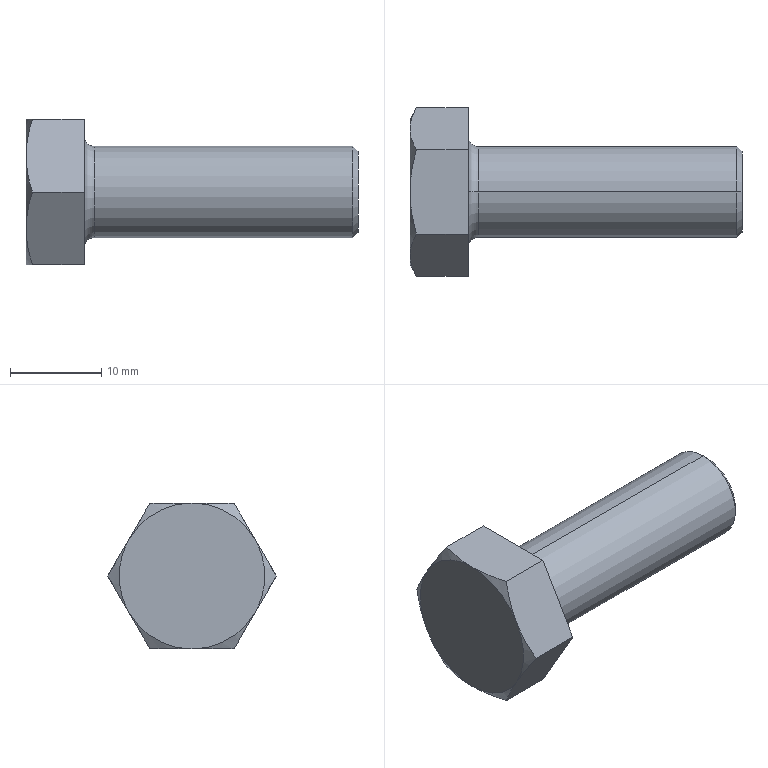Part | SolidWorks | features Chamfer 2, RevCut 2, Revolution 2, Extrusion 1, ICE 1 | 1 solid | 21 faces | box 36.4 x 18.475 x 16 mm | volume 3775 mm3 | plane 9 | cone 8 | cylinder 2 | torus 2 | commonest cylinder face diameters 10 x2
STEP:
#1=CARTESIAN_POINT('',(36.4,0.,-4.444));
#2=VERTEX_POINT('',#1);
#3=CARTESIAN_POINT('',(36.4,0.,4.444));
#4=VERTEX_POINT('',#3);
#5=CARTESIAN_POINT('',(36.4,0.,0.));
#6=DIRECTION('',(1.,0.,0.));
#7=DIRECTION('',(0.,0.,1.));
#8=AXIS2_PLACEMENT_3D('',#5,#6,#7);
#9=CIRCLE('',#8,4.444);
#10=EDGE_CURVE('',#2,#4,#9,.T.);
#11=ORIENTED_EDGE('',*,*,#10,.F.);
#12=CARTESIAN_POINT('',(35.844,0.,-5.));
#13=VERTEX_POINT('',#12);
#14=CARTESIAN_POINT('',(35.844,0.,-5.));
#15=DIRECTION('',(-0.7071,0.,-0.7071));
#16=VECTOR('',#15,1000.);
#17=LINE('',#14,#16);
#18=EDGE_CURVE('',#2,#13,#17,.T.);
#19=ORIENTED_EDGE('',*,*,#18,.T.);
#20=CARTESIAN_POINT('',(35.844,0.,5.));
#21=VERTEX_POINT('',#20);
#22=CARTESIAN_POINT('',(35.844,0.,0.));
#23=DIRECTION('',(-1.,0.,0.));
#24=DIRECTION('',(0.,0.,1.));
#25=AXIS2_PLACEMENT_3D('',#22,#23,#24);
#26=CIRCLE('',#25,5.);
#27=EDGE_CURVE('',#21,#13,#26,.T.);
#28=ORIENTED_EDGE('',*,*,#27,.F.);
#29=CARTESIAN_POINT('',(35.844,0.,5.));
#30=DIRECTION('',(-0.7071,0.,0.7071));
#31=VECTOR('',#30,1000.);
#32=LINE('',#29,#31);
#33=EDGE_CURVE('',#4,#21,#32,.T.);
#34=ORIENTED_EDGE('',*,*,#33,.F.);
#35=EDGE_LOOP('',(#11,#19,#28,#34));
#36=FACE_OUTER_BOUND('',#35,.T.);
#37=CARTESIAN_POINT('',(35.844,0.,0.));
#38=DIRECTION('',(-1.,0.,0.));
#39=DIRECTION('',(0.,0.,1.));
#40=AXIS2_PLACEMENT_3D('',#37,#38,#39);
#41=CONICAL_SURFACE('',#40,5.,0.7854);
#42=ADVANCED_FACE('',(#36),#41,.T.);
#43=ORIENTED_EDGE('',*,*,#27,.T.);
#44=CARTESIAN_POINT('',(7.5,0.,-5.));
#45=VERTEX_POINT('',#44);
#46=CARTESIAN_POINT('',(6.4,0.,-5.));
#47=DIRECTION('',(-1.,0.,0.));
#48=VECTOR('',#47,1000.);
#49=LINE('',#46,#48);
#50=EDGE_CURVE('',#13,#45,#49,.T.);
#51=ORIENTED_EDGE('',*,*,#50,.T.);
#52=CARTESIAN_POINT('',(7.5,0.,5.));
#53=VERTEX_POINT('',#52);
#54=CARTESIAN_POINT('',(7.5,0.,0.));
#55=DIRECTION('',(-1.,0.,0.));
#56=DIRECTION('',(0.,0.,1.));
#57=AXIS2_PLACEMENT_3D('',#54,#55,#56);
#58=CIRCLE('',#57,5.);
#59=EDGE_CURVE('',#53,#45,#58,.T.);
#60=ORIENTED_EDGE('',*,*,#59,.F.);
#61=CARTESIAN_POINT('',(6.4,0.,5.));
#62=DIRECTION('',(-1.,0.,0.));
#63=VECTOR('',#62,1000.);
#64=LINE('',#61,#63);
#65=EDGE_CURVE('',#21,#53,#64,.T.);
#66=ORIENTED_EDGE('',*,*,#65,.F.);
#67=EDGE_LOOP('',(#43,#51,#60,#66));
#68=FACE_OUTER_BOUND('',#67,.T.);
#69=CARTESIAN_POINT('',(6.4,0.,0.));
#70=DIRECTION('',(-1.,0.,0.));
#71=DIRECTION('',(0.,0.,1.));
#72=AXIS2_PLACEMENT_3D('',#69,#70,#71);
#73=CYLINDRICAL_SURFACE('',#72,5.);
#74=ADVANCED_FACE('',(#68),#73,.T.);
#75=CARTESIAN_POINT('',(6.4,0.,-6.1));
#76=VERTEX_POINT('',#75);
#77=CARTESIAN_POINT('',(6.4,0.,6.1));
#78=VERTEX_POINT('',#77);
#79=CARTESIAN_POINT('',(6.4,0.,0.));
#80=DIRECTION('',(-1.,0.,0.));
#81=DIRECTION('',(0.,0.,1.));
#82=AXIS2_PLACEMENT_3D('',#79,#80,#81);
#83=CIRCLE('',#82,6.1);
#84=EDGE_CURVE('',#76,#78,#83,.T.);
#85=ORIENTED_EDGE('',*,*,#84,.F.);
#86=CARTESIAN_POINT('',(7.5,0.,-6.1));
#87=DIRECTION('',(0.,1.,0.));
#88=DIRECTION('',(0.,0.,1.));
#89=AXIS2_PLACEMENT_3D('',#86,#87,#88);
#90=CIRCLE('',#89,1.1);
#91=EDGE_CURVE('',#76,#45,#90,.T.);
#92=ORIENTED_EDGE('',*,*,#91,.T.);
#93=CARTESIAN_POINT('',(7.5,0.,0.));
#94=DIRECTION('',(-1.,0.,0.));
#95=DIRECTION('',(0.,0.,1.));
#96=AXIS2_PLACEMENT_3D('',#93,#94,#95);
#97=CIRCLE('',#96,5.);
#98=EDGE_CURVE('',#45,#53,#97,.T.);
#99=ORIENTED_EDGE('',*,*,#98,.T.);
#100=CARTESIAN_POINT('',(7.5,0.,6.1));
#101=DIRECTION('',(0.,-1.,0.));
#102=DIRECTION('',(0.,0.,-1.));
#103=AXIS2_PLACEMENT_3D('',#100,#101,#102);
#104=CIRCLE('',#103,1.1);
#105=EDGE_CURVE('',#78,#53,#104,.T.);
#106=ORIENTED_EDGE('',*,*,#105,.F.);
#107=EDGE_LOOP('',(#85,#92,#99,#106));
#108=FACE_OUTER_BOUND('',#107,.T.);
#109=CARTESIAN_POINT('',(7.5,0.,0.));
#110=DIRECTION('',(-1.,0.,0.));
#111=DIRECTION('',(0.,0.,1.));
#112=AXIS2_PLACEMENT_3D('',#109,#110,#111);
#113=TOROIDAL_SURFACE('',#112,6.1,1.1);
#114=ADVANCED_FACE('',(#108),#113,.F.);
#115=CARTESIAN_POINT('',(6.4,-4.619,-8.));
#116=VERTEX_POINT('',#115);
#117=CARTESIAN_POINT('',(6.4,4.619,-8.));
#118=VERTEX_POINT('',#117);
#119=CARTESIAN_POINT('',(6.4,-4.619,-8.));
#120=DIRECTION('',(0.,1.,0.));
#121=VECTOR('',#120,1000.);
#122=LINE('',#119,#121);
#123=EDGE_CURVE('',#116,#118,#122,.T.);
#124=ORIENTED_EDGE('',*,*,#123,.T.);
#125=CARTESIAN_POINT('',(6.4,9.238,0.));
#126=VERTEX_POINT('',#125);
#127=CARTESIAN_POINT('',(6.4,4.619,-8.));
#128=DIRECTION('',(0.,0.5,0.866));
#129=VECTOR('',#128,1000.);
#130=LINE('',#127,#129);
#131=EDGE_CURVE('',#118,#126,#130,.T.);
#132=ORIENTED_EDGE('',*,*,#131,.T.);
#133=CARTESIAN_POINT('',(6.4,4.619,8.));
#134=VERTEX_POINT('',#133);
#135=CARTESIAN_POINT('',(6.4,9.238,0.));
#136=DIRECTION('',(0.,-0.5,0.866));
#137=VECTOR('',#136,1000.);
#138=LINE('',#135,#137);
#139=EDGE_CURVE('',#126,#134,#138,.T.);
#140=ORIENTED_EDGE('',*,*,#139,.T.);
#141=CARTESIAN_POINT('',(6.4,-4.619,8.));
#142=VERTEX_POINT('',#141);
#143=CARTESIAN_POINT('',(6.4,4.619,8.));
#144=DIRECTION('',(0.,-1.,0.));
#145=VECTOR('',#144,1000.);
#146=LINE('',#143,#145);
#147=EDGE_CURVE('',#134,#142,#146,.T.);
#148=ORIENTED_EDGE('',*,*,#147,.T.);
#149=CARTESIAN_POINT('',(6.4,-9.238,0.));
#150=VERTEX_POINT('',#149);
#151=CARTESIAN_POINT('',(6.4,-4.619,8.));
#152=DIRECTION('',(0.,-0.5,-0.866));
#153=VECTOR('',#152,1000.);
#154=LINE('',#151,#153);
#155=EDGE_CURVE('',#142,#150,#154,.T.);
#156=ORIENTED_EDGE('',*,*,#155,.T.);
#157=CARTESIAN_POINT('',(6.4,-9.238,0.));
#158=DIRECTION('',(0.,0.5,-0.866));
#159=VECTOR('',#158,1000.);
#160=LINE('',#157,#159);
#161=EDGE_CURVE('',#150,#116,#160,.T.);
#162=ORIENTED_EDGE('',*,*,#161,.T.);
#163=EDGE_LOOP('',(#124,#132,#140,#148,#156,#162));
#164=FACE_OUTER_BOUND('',#163,.T.);
#165=CARTESIAN_POINT('',(6.4,0.,0.));
#166=DIRECTION('',(-1.,0.,0.));
#167=DIRECTION('',(0.,0.,1.));
#168=AXIS2_PLACEMENT_3D('',#165,#166,#167);
#169=CIRCLE('',#168,6.1);
#170=EDGE_CURVE('',#78,#76,#169,.T.);
#171=ORIENTED_EDGE('',*,*,#170,.T.);
#172=ORIENTED_EDGE('',*,*,#84,.T.);
#173=EDGE_LOOP('',(#171,#172));
#174=FACE_BOUND('',#173,.T.);
#175=CARTESIAN_POINT('',(6.4,4.619,-8.));
#176=DIRECTION('',(1.,0.,0.));
#177=DIRECTION('',(0.,0.,-1.));
#178=AXIS2_PLACEMENT_3D('',#175,#176,#177);
#179=PLANE('',#178);
#180=ADVANCED_FACE('',(#164,#174),#179,.T.);
#181=CARTESIAN_POINT('',(0.7145,4.619,-8.));
#182=VERTEX_POINT('',#181);
#183=CARTESIAN_POINT('',(0.,0.,-8.));
#184=VERTEX_POINT('',#183);
#185=CARTESIAN_POINT('',(0.7145,4.619,-8.));
#186=CARTESIAN_POINT('',(0.4989,3.872,-8.));
#187=CARTESIAN_POINT('',(0.3194,3.115,-8.));
#188=CARTESIAN_POINT('',(0.06895,1.573,-8.));
#189=CARTESIAN_POINT('',(0.,0.781,-8.));
#190=CARTESIAN_POINT('',(0.,0.,-8.));
#191=B_SPLINE_CURVE_WITH_KNOTS('',3,(#185,#186,#187,#188,#189,#190),.UNSPECIFIED.,.F.,.F.,(4,2,4),(0.003372,0.005703,0.008035),.UNSPECIFIED.);
#192=EDGE_CURVE('',#182,#184,#191,.T.);
#193=ORIENTED_EDGE('',*,*,#192,.F.);
#194=CARTESIAN_POINT('',(6.4,4.619,-8.));
#195=DIRECTION('',(-1.,0.,0.));
#196=VECTOR('',#195,1000.);
#197=LINE('',#194,#196);
#198=EDGE_CURVE('',#118,#182,#197,.T.);
#199=ORIENTED_EDGE('',*,*,#198,.F.);
#200=ORIENTED_EDGE('',*,*,#123,.F.);
#201=CARTESIAN_POINT('',(0.7145,-4.619,-8.));
#202=VERTEX_POINT('',#201);
#203=CARTESIAN_POINT('',(6.4,-4.619,-8.));
#204=DIRECTION('',(-1.,0.,0.));
#205=VECTOR('',#204,1000.);
#206=LINE('',#203,#205);
#207=EDGE_CURVE('',#116,#202,#206,.T.);
#208=ORIENTED_EDGE('',*,*,#207,.T.);
#209=CARTESIAN_POINT('',(0.,0.,-8.));
#210=CARTESIAN_POINT('',(0.,-0.7805,-8.));
#211=CARTESIAN_POINT('',(0.06709,-1.556,-8.));
#212=CARTESIAN_POINT('',(0.3158,-3.098,-8.));
#213=CARTESIAN_POINT('',(0.4977,-3.868,-8.));
#214=CARTESIAN_POINT('',(0.7145,-4.619,-8.));
#215=B_SPLINE_CURVE_WITH_KNOTS('',3,(#209,#210,#211,#212,#213,#214),.UNSPECIFIED.,.F.,.F.,(4,2,4),(0.008035,0.01037,0.0127),.UNSPECIFIED.);
#216=EDGE_CURVE('',#184,#202,#215,.T.);
#217=ORIENTED_EDGE('',*,*,#216,.F.);
#218=EDGE_LOOP('',(#193,#199,#200,#208,#217));
#219=FACE_OUTER_BOUND('',#218,.T.);
#220=CARTESIAN_POINT('',(6.4,-4.619,-8.));
#221=DIRECTION('',(0.,0.,1.));
#222=DIRECTION('',(1.,0.,0.));
#223=AXIS2_PLACEMENT_3D('',#220,#221,#222);
#224=PLANE('',#223);
#225=ADVANCED_FACE('',(#219),#224,.F.);
#226=CARTESIAN_POINT('',(0.7145,9.238,0.));
#227=VERTEX_POINT('',#226);
#228=CARTESIAN_POINT('',(0.,6.928,-4.));
#229=VERTEX_POINT('',#228);
#230=CARTESIAN_POINT('',(0.7145,9.238,0.));
#231=CARTESIAN_POINT('',(0.4964,8.86,-0.6543));
#232=CARTESIAN_POINT('',(0.3167,8.479,-1.313));
#233=CARTESIAN_POINT('',(0.0681,7.71,-2.646));
#234=CARTESIAN_POINT('',(0.,7.322,-3.319));
#235=CARTESIAN_POINT('',(0.,6.928,-4.));
#236=B_SPLINE_CURVE_WITH_KNOTS('',3,(#230,#231,#232,#233,#234,#235),.UNSPECIFIED.,.F.,.F.,(4,2,4),(0.000000238,0.002337,0.004674),.UNSPECIFIED.);
#237=EDGE_CURVE('',#227,#229,#236,.T.);
#238=ORIENTED_EDGE('',*,*,#237,.F.);
#239=CARTESIAN_POINT('',(6.4,9.238,0.));
#240=DIRECTION('',(-1.,0.,0.));
#241=VECTOR('',#240,1000.);
#242=LINE('',#239,#241);
#243=EDGE_CURVE('',#126,#227,#242,.T.);
#244=ORIENTED_EDGE('',*,*,#243,.F.);
#245=ORIENTED_EDGE('',*,*,#131,.F.);
#246=ORIENTED_EDGE('',*,*,#198,.T.);
#247=CARTESIAN_POINT('',(0.,6.928,-4.));
#248=CARTESIAN_POINT('',(0.,6.732,-4.339));
#249=CARTESIAN_POINT('',(0.01689,6.535,-4.68));
#250=CARTESIAN_POINT('',(0.08225,6.146,-5.355));
#251=CARTESIAN_POINT('',(0.1307,5.952,-5.69));
#252=CARTESIAN_POINT('',(0.3174,5.376,-6.689));
#253=CARTESIAN_POINT('',(0.497,4.996,-7.347));
#254=CARTESIAN_POINT('',(0.7145,4.619,-8.));
#255=B_SPLINE_CURVE_WITH_KNOTS('',3,(#247,#248,#249,#250,#251,#252,#253,#254),.UNSPECIFIED.,.F.,.F.,(4,2,2,4),(0.004674,0.005838,0.007002,0.00933),.UNSPECIFIED.);
#256=EDGE_CURVE('',#229,#182,#255,.T.);
#257=ORIENTED_EDGE('',*,*,#256,.F.);
#258=EDGE_LOOP('',(#238,#244,#245,#246,#257));
#259=FACE_OUTER_BOUND('',#258,.T.);
#260=CARTESIAN_POINT('',(6.4,4.619,-8.));
#261=DIRECTION('',(0.,-0.866,0.5));
#262=DIRECTION('',(0.,-0.5,-0.866));
#263=AXIS2_PLACEMENT_3D('',#260,#261,#262);
#264=PLANE('',#263);
#265=ADVANCED_FACE('',(#259),#264,.F.);
#266=CARTESIAN_POINT('',(0.7145,4.619,8.));
#267=VERTEX_POINT('',#266);
#268=CARTESIAN_POINT('',(0.,6.928,4.));
#269=VERTEX_POINT('',#268);
#270=CARTESIAN_POINT('',(0.7145,4.619,8.));
#271=CARTESIAN_POINT('',(0.4964,4.997,7.346));
#272=CARTESIAN_POINT('',(0.3167,5.377,6.687));
#273=CARTESIAN_POINT('',(0.0681,6.146,5.354));
#274=CARTESIAN_POINT('',(0.,6.535,4.681));
#275=CARTESIAN_POINT('',(0.,6.928,4.));
#276=B_SPLINE_CURVE_WITH_KNOTS('',3,(#270,#271,#272,#273,#274,#275),.UNSPECIFIED.,.F.,.F.,(4,2,4),(0.000000238,0.002337,0.004674),.UNSPECIFIED.);
#277=EDGE_CURVE('',#267,#269,#276,.T.);
#278=ORIENTED_EDGE('',*,*,#277,.F.);
#279=CARTESIAN_POINT('',(6.4,4.619,8.));
#280=DIRECTION('',(-1.,0.,0.));
#281=VECTOR('',#280,1000.);
#282=LINE('',#279,#281);
#283=EDGE_CURVE('',#134,#267,#282,.T.);
#284=ORIENTED_EDGE('',*,*,#283,.F.);
#285=ORIENTED_EDGE('',*,*,#139,.F.);
#286=ORIENTED_EDGE('',*,*,#243,.T.);
#287=CARTESIAN_POINT('',(0.,6.928,4.));
#288=CARTESIAN_POINT('',(0.,7.124,3.661));
#289=CARTESIAN_POINT('',(0.01689,7.321,3.32));
#290=CARTESIAN_POINT('',(0.08225,7.711,2.645));
#291=CARTESIAN_POINT('',(0.1307,7.904,2.31));
#292=CARTESIAN_POINT('',(0.3174,8.481,1.311));
#293=CARTESIAN_POINT('',(0.497,8.861,0.6527));
#294=CARTESIAN_POINT('',(0.7145,9.238,0.));
#295=B_SPLINE_CURVE_WITH_KNOTS('',3,(#287,#288,#289,#290,#291,#292,#293,#294),.UNSPECIFIED.,.F.,.F.,(4,2,2,4),(0.004674,0.005838,0.007002,0.00933),.UNSPECIFIED.);
#296=EDGE_CURVE('',#269,#227,#295,.T.);
#297=ORIENTED_EDGE('',*,*,#296,.F.);
#298=EDGE_LOOP('',(#278,#284,#285,#286,#297));
#299=FACE_OUTER_BOUND('',#298,.T.);
#300=CARTESIAN_POINT('',(6.4,9.238,0.));
#301=DIRECTION('',(0.,-0.866,-0.5));
#302=DIRECTION('',(0.,0.5,-0.866));
#303=AXIS2_PLACEMENT_3D('',#300,#301,#302);
#304=PLANE('',#303);
#305=ADVANCED_FACE('',(#299),#304,.F.);
#306=CARTESIAN_POINT('',(0.7145,-4.619,8.));
#307=VERTEX_POINT('',#306);
#308=CARTESIAN_POINT('',(0.,0.,8.));
#309=VERTEX_POINT('',#308);
#310=CARTESIAN_POINT('',(0.7145,-4.619,8.));
#311=CARTESIAN_POINT('',(0.4977,-3.868,8.));
#312=CARTESIAN_POINT('',(0.3158,-3.098,8.));
#313=CARTESIAN_POINT('',(0.06709,-1.556,8.));
#314=CARTESIAN_POINT('',(0.,-0.7805,8.));
#315=CARTESIAN_POINT('',(0.,0.,8.));
#316=B_SPLINE_CURVE_WITH_KNOTS('',3,(#310,#311,#312,#313,#314,#315),.UNSPECIFIED.,.F.,.F.,(4,2,4),(0.008254,0.01059,0.01293),.UNSPECIFIED.);
#317=EDGE_CURVE('',#307,#309,#316,.T.);
#318=ORIENTED_EDGE('',*,*,#317,.F.);
#319=CARTESIAN_POINT('',(6.4,-4.619,8.));
#320=DIRECTION('',(-1.,0.,0.));
#321=VECTOR('',#320,1000.);
#322=LINE('',#319,#321);
#323=EDGE_CURVE('',#142,#307,#322,.T.);
#324=ORIENTED_EDGE('',*,*,#323,.F.);
#325=ORIENTED_EDGE('',*,*,#147,.F.);
#326=ORIENTED_EDGE('',*,*,#283,.T.);
#327=CARTESIAN_POINT('',(0.,0.,8.));
#328=CARTESIAN_POINT('',(0.,0.781,8.));
#329=CARTESIAN_POINT('',(0.06895,1.573,8.));
#330=CARTESIAN_POINT('',(0.3194,3.115,8.));
#331=CARTESIAN_POINT('',(0.4989,3.872,8.));
#332=CARTESIAN_POINT('',(0.7145,4.619,8.));
#333=B_SPLINE_CURVE_WITH_KNOTS('',3,(#327,#328,#329,#330,#331,#332),.UNSPECIFIED.,.F.,.F.,(4,2,4),(0.01293,0.01526,0.0176),.UNSPECIFIED.);
#334=EDGE_CURVE('',#309,#267,#333,.T.);
#335=ORIENTED_EDGE('',*,*,#334,.F.);
#336=EDGE_LOOP('',(#318,#324,#325,#326,#335));
#337=FACE_OUTER_BOUND('',#336,.T.);
#338=CARTESIAN_POINT('',(6.4,4.619,8.));
#339=DIRECTION('',(0.,0.,-1.));
#340=DIRECTION('',(0.,1.,0.));
#341=AXIS2_PLACEMENT_3D('',#338,#339,#340);
#342=PLANE('',#341);
#343=ADVANCED_FACE('',(#337),#342,.F.);
#344=CARTESIAN_POINT('',(0.7145,-9.238,0.));
#345=VERTEX_POINT('',#344);
#346=CARTESIAN_POINT('',(0.,-6.928,4.));
#347=VERTEX_POINT('',#346);
#348=CARTESIAN_POINT('',(0.7145,-9.238,0.));
#349=CARTESIAN_POINT('',(0.4964,-8.86,0.6543));
#350=CARTESIAN_POINT('',(0.3167,-8.479,1.313));
#351=CARTESIAN_POINT('',(0.0681,-7.71,2.646));
#352=CARTESIAN_POINT('',(0.,-7.322,3.319));
#353=CARTESIAN_POINT('',(0.,-6.928,4.));
#354=B_SPLINE_CURVE_WITH_KNOTS('',3,(#348,#349,#350,#351,#352,#353),.UNSPECIFIED.,.F.,.F.,(4,2,4),(0.000000238,0.002337,0.004674),.UNSPECIFIED.);
#355=EDGE_CURVE('',#345,#347,#354,.T.);
#356=ORIENTED_EDGE('',*,*,#355,.F.);
#357=CARTESIAN_POINT('',(6.4,-9.238,0.));
#358=DIRECTION('',(-1.,0.,0.));
#359=VECTOR('',#358,1000.);
#360=LINE('',#357,#359);
#361=EDGE_CURVE('',#150,#345,#360,.T.);
#362=ORIENTED_EDGE('',*,*,#361,.F.);
#363=ORIENTED_EDGE('',*,*,#155,.F.);
#364=ORIENTED_EDGE('',*,*,#323,.T.);
#365=CARTESIAN_POINT('',(0.,-6.928,4.));
#366=CARTESIAN_POINT('',(0.,-6.732,4.339));
#367=CARTESIAN_POINT('',(0.01689,-6.535,4.68));
#368=CARTESIAN_POINT('',(0.08225,-6.146,5.355));
#369=CARTESIAN_POINT('',(0.1307,-5.952,5.69));
#370=CARTESIAN_POINT('',(0.3174,-5.376,6.689));
#371=CARTESIAN_POINT('',(0.497,-4.996,7.347));
#372=CARTESIAN_POINT('',(0.7145,-4.619,8.));
#373=B_SPLINE_CURVE_WITH_KNOTS('',3,(#365,#366,#367,#368,#369,#370,#371,#372),.UNSPECIFIED.,.F.,.F.,(4,2,2,4),(0.004674,0.005838,0.007002,0.00933),.UNSPECIFIED.);
#374=EDGE_CURVE('',#347,#307,#373,.T.);
#375=ORIENTED_EDGE('',*,*,#374,.F.);
#376=EDGE_LOOP('',(#356,#362,#363,#364,#375));
#377=FACE_OUTER_BOUND('',#376,.T.);
#378=CARTESIAN_POINT('',(6.4,-4.619,8.));
#379=DIRECTION('',(0.,0.866,-0.5));
#380=DIRECTION('',(0.,0.5,0.866));
#381=AXIS2_PLACEMENT_3D('',#378,#379,#380);
#382=PLANE('',#381);
#383=ADVANCED_FACE('',(#377),#382,.F.);
#384=CARTESIAN_POINT('',(0.,-6.928,-4.));
#385=VERTEX_POINT('',#384);
#386=CARTESIAN_POINT('',(0.7145,-4.619,-8.));
#387=CARTESIAN_POINT('',(0.4964,-4.997,-7.346));
#388=CARTESIAN_POINT('',(0.3167,-5.377,-6.687));
#389=CARTESIAN_POINT('',(0.0681,-6.146,-5.354));
#390=CARTESIAN_POINT('',(0.,-6.535,-4.681));
#391=CARTESIAN_POINT('',(0.,-6.928,-4.));
#392=B_SPLINE_CURVE_WITH_KNOTS('',3,(#386,#387,#388,#389,#390,#391),.UNSPECIFIED.,.F.,.F.,(4,2,4),(0.000000238,0.002337,0.004674),.UNSPECIFIED.);
#393=EDGE_CURVE('',#202,#385,#392,.T.);
#394=ORIENTED_EDGE('',*,*,#393,.F.);
#395=ORIENTED_EDGE('',*,*,#207,.F.);
#396=ORIENTED_EDGE('',*,*,#161,.F.);
#397=ORIENTED_EDGE('',*,*,#361,.T.);
#398=CARTESIAN_POINT('',(0.,-6.928,-4.));
#399=CARTESIAN_POINT('',(0.,-7.124,-3.661));
#400=CARTESIAN_POINT('',(0.01689,-7.321,-3.32));
#401=CARTESIAN_POINT('',(0.08225,-7.711,-2.645));
#402=CARTESIAN_POINT('',(0.1307,-7.904,-2.31));
#403=CARTESIAN_POINT('',(0.3174,-8.481,-1.311));
#404=CARTESIAN_POINT('',(0.497,-8.861,-0.6527));
#405=CARTESIAN_POINT('',(0.7145,-9.238,0.));
#406=B_SPLINE_CURVE_WITH_KNOTS('',3,(#398,#399,#400,#401,#402,#403,#404,#405),.UNSPECIFIED.,.F.,.F.,(4,2,2,4),(0.004674,0.005838,0.007002,0.00933),.UNSPECIFIED.);
#407=EDGE_CURVE('',#385,#345,#406,.T.);
#408=ORIENTED_EDGE('',*,*,#407,.F.);
#409=EDGE_LOOP('',(#394,#395,#396,#397,#408));
#410=FACE_OUTER_BOUND('',#409,.T.);
#411=CARTESIAN_POINT('',(6.4,-9.238,0.));
#412=DIRECTION('',(0.,0.866,0.5));
#413=DIRECTION('',(0.,-0.5,0.866));
#414=AXIS2_PLACEMENT_3D('',#411,#412,#413);
#415=PLANE('',#414);
#416=ADVANCED_FACE('',(#410),#415,.F.);
#417=ORIENTED_EDGE('',*,*,#216,.T.);
#418=ORIENTED_EDGE('',*,*,#393,.T.);
#419=CARTESIAN_POINT('',(0.,0.,0.));
#420=DIRECTION('',(1.,0.,0.));
#421=DIRECTION('',(0.,0.,-1.));
#422=AXIS2_PLACEMENT_3D('',#419,#420,#421);
#423=CIRCLE('',#422,8.);
#424=EDGE_CURVE('',#385,#184,#423,.T.);
#425=ORIENTED_EDGE('',*,*,#424,.T.);
#426=EDGE_LOOP('',(#417,#418,#425));
#427=FACE_OUTER_BOUND('',#426,.T.);
#428=CARTESIAN_POINT('',(0.,0.,0.));
#429=DIRECTION('',(1.,0.,0.));
#430=DIRECTION('',(0.,0.,1.));
#431=AXIS2_PLACEMENT_3D('',#428,#429,#430);
#432=CONICAL_SURFACE('',#431,8.,1.047);
#433=ADVANCED_FACE('',(#427),#432,.T.);
#434=ORIENTED_EDGE('',*,*,#355,.T.);
#435=CARTESIAN_POINT('',(0.,0.,0.));
#436=DIRECTION('',(1.,0.,0.));
#437=DIRECTION('',(0.,0.,-1.));
#438=AXIS2_PLACEMENT_3D('',#435,#436,#437);
#439=CIRCLE('',#438,8.);
#440=EDGE_CURVE('',#347,#385,#439,.T.);
#441=ORIENTED_EDGE('',*,*,#440,.T.);
#442=ORIENTED_EDGE('',*,*,#407,.T.);
#443=EDGE_LOOP('',(#434,#441,#442));
#444=FACE_OUTER_BOUND('',#443,.T.);
#445=CARTESIAN_POINT('',(0.,0.,0.));
#446=DIRECTION('',(1.,0.,0.));
#447=DIRECTION('',(0.,0.,1.));
#448=AXIS2_PLACEMENT_3D('',#445,#446,#447);
#449=CONICAL_SURFACE('',#448,8.,1.047);
#450=ADVANCED_FACE('',(#444),#449,.T.);
#451=ORIENTED_EDGE('',*,*,#317,.T.);
#452=CARTESIAN_POINT('',(0.,0.,0.));
#453=DIRECTION('',(1.,0.,0.));
#454=DIRECTION('',(0.,0.,-1.));
#455=AXIS2_PLACEMENT_3D('',#452,#453,#454);
#456=CIRCLE('',#455,8.);
#457=EDGE_CURVE('',#309,#347,#456,.T.);
#458=ORIENTED_EDGE('',*,*,#457,.T.);
#459=ORIENTED_EDGE('',*,*,#374,.T.);
#460=EDGE_LOOP('',(#451,#458,#459));
#461=FACE_OUTER_BOUND('',#460,.T.);
#462=CARTESIAN_POINT('',(0.,0.,0.));
#463=DIRECTION('',(1.,0.,0.));
#464=DIRECTION('',(0.,0.,1.));
#465=AXIS2_PLACEMENT_3D('',#462,#463,#464);
#466=CONICAL_SURFACE('',#465,8.,1.047);
#467=ADVANCED_FACE('',(#461),#466,.T.);
#468=ORIENTED_EDGE('',*,*,#277,.T.);
#469=CARTESIAN_POINT('',(0.,0.,0.));
#470=DIRECTION('',(-1.,0.,0.));
#471=DIRECTION('',(0.,0.,1.));
#472=AXIS2_PLACEMENT_3D('',#469,#470,#471);
#473=CIRCLE('',#472,8.);
#474=EDGE_CURVE('',#309,#269,#473,.T.);
#475=ORIENTED_EDGE('',*,*,#474,.F.);
#476=ORIENTED_EDGE('',*,*,#334,.T.);
#477=EDGE_LOOP('',(#468,#475,#476));
#478=FACE_OUTER_BOUND('',#477,.T.);
#479=CARTESIAN_POINT('',(0.,0.,0.));
#480=DIRECTION('',(1.,0.,0.));
#481=DIRECTION('',(0.,0.,1.));
#482=AXIS2_PLACEMENT_3D('',#479,#480,#481);
#483=CONICAL_SURFACE('',#482,8.,1.047);
#484=ADVANCED_FACE('',(#478),#483,.T.);
#485=ORIENTED_EDGE('',*,*,#296,.T.);
#486=ORIENTED_EDGE('',*,*,#237,.T.);
#487=CARTESIAN_POINT('',(0.,0.,0.));
#488=DIRECTION('',(1.,0.,0.));
#489=DIRECTION('',(0.,0.,-1.));
#490=AXIS2_PLACEMENT_3D('',#487,#488,#489);
#491=CIRCLE('',#490,8.);
#492=EDGE_CURVE('',#229,#269,#491,.T.);
#493=ORIENTED_EDGE('',*,*,#492,.T.);
#494=EDGE_LOOP('',(#485,#486,#493));
#495=FACE_OUTER_BOUND('',#494,.T.);
#496=CARTESIAN_POINT('',(0.,0.,0.));
#497=DIRECTION('',(1.,0.,0.));
#498=DIRECTION('',(0.,0.,1.));
#499=AXIS2_PLACEMENT_3D('',#496,#497,#498);
#500=CONICAL_SURFACE('',#499,8.,1.047);
#501=ADVANCED_FACE('',(#495),#500,.T.);
#502=ORIENTED_EDGE('',*,*,#256,.T.);
#503=ORIENTED_EDGE('',*,*,#192,.T.);
#504=CARTESIAN_POINT('',(0.,0.,0.));
#505=DIRECTION('',(1.,0.,0.));
#506=DIRECTION('',(0.,0.,-1.));
#507=AXIS2_PLACEMENT_3D('',#504,#505,#506);
#508=CIRCLE('',#507,8.);
#509=EDGE_CURVE('',#184,#229,#508,.T.);
#510=ORIENTED_EDGE('',*,*,#509,.T.);
#511=EDGE_LOOP('',(#502,#503,#510));
#512=FACE_OUTER_BOUND('',#511,.T.);
#513=CARTESIAN_POINT('',(0.,0.,0.));
#514=DIRECTION('',(1.,0.,0.));
#515=DIRECTION('',(0.,0.,1.));
#516=AXIS2_PLACEMENT_3D('',#513,#514,#515);
#517=CONICAL_SURFACE('',#516,8.,1.047);
#518=ADVANCED_FACE('',(#512),#517,.T.);
#519=ORIENTED_EDGE('',*,*,#509,.F.);
#520=ORIENTED_EDGE('',*,*,#424,.F.);
#521=ORIENTED_EDGE('',*,*,#440,.F.);
#522=ORIENTED_EDGE('',*,*,#457,.F.);
#523=ORIENTED_EDGE('',*,*,#474,.T.);
#524=ORIENTED_EDGE('',*,*,#492,.F.);
#525=EDGE_LOOP('',(#519,#520,#521,#522,#523,#524));
#526=FACE_OUTER_BOUND('',#525,.T.);
#527=CARTESIAN_POINT('',(0.,4.619,-8.));
#528=DIRECTION('',(1.,0.,0.));
#529=DIRECTION('',(0.,0.,-1.));
#530=AXIS2_PLACEMENT_3D('',#527,#528,#529);
#531=PLANE('',#530);
#532=ADVANCED_FACE('',(#526),#531,.F.);
#533=ORIENTED_EDGE('',*,*,#91,.F.);
#534=ORIENTED_EDGE('',*,*,#170,.F.);
#535=ORIENTED_EDGE('',*,*,#105,.T.);
#536=ORIENTED_EDGE('',*,*,#59,.T.);
#537=EDGE_LOOP('',(#533,#534,#535,#536));
#538=FACE_OUTER_BOUND('',#537,.T.);
#539=CARTESIAN_POINT('',(7.5,0.,0.));
#540=DIRECTION('',(-1.,0.,0.));
#541=DIRECTION('',(0.,0.,1.));
#542=AXIS2_PLACEMENT_3D('',#539,#540,#541);
#543=TOROIDAL_SURFACE('',#542,6.1,1.1);
#544=ADVANCED_FACE('',(#538),#543,.F.);
#545=CARTESIAN_POINT('',(36.4,0.,0.));
#546=DIRECTION('',(1.,0.,0.));
#547=DIRECTION('',(0.,0.,1.));
#548=AXIS2_PLACEMENT_3D('',#545,#546,#547);
#549=CIRCLE('',#548,4.444);
#550=EDGE_CURVE('',#4,#2,#549,.T.);
#551=ORIENTED_EDGE('',*,*,#550,.T.);
#552=ORIENTED_EDGE('',*,*,#10,.T.);
#553=EDGE_LOOP('',(#551,#552));
#554=FACE_OUTER_BOUND('',#553,.T.);
#555=CARTESIAN_POINT('',(36.4,5.,0.));
#556=DIRECTION('',(-1.,0.,0.));
#557=DIRECTION('',(0.,0.,1.));
#558=AXIS2_PLACEMENT_3D('',#555,#556,#557);
#559=PLANE('',#558);
#560=ADVANCED_FACE('',(#554),#559,.F.);
#561=ORIENTED_EDGE('',*,*,#50,.F.);
#562=CARTESIAN_POINT('',(35.844,0.,0.));
#563=DIRECTION('',(-1.,0.,0.));
#564=DIRECTION('',(0.,0.,1.));
#565=AXIS2_PLACEMENT_3D('',#562,#563,#564);
#566=CIRCLE('',#565,5.);
#567=EDGE_CURVE('',#13,#21,#566,.T.);
#568=ORIENTED_EDGE('',*,*,#567,.T.);
#569=ORIENTED_EDGE('',*,*,#65,.T.);
#570=ORIENTED_EDGE('',*,*,#98,.F.);
#571=EDGE_LOOP('',(#561,#568,#569,#570));
#572=FACE_OUTER_BOUND('',#571,.T.);
#573=CARTESIAN_POINT('',(6.4,0.,0.));
#574=DIRECTION('',(-1.,0.,0.));
#575=DIRECTION('',(0.,0.,1.));
#576=AXIS2_PLACEMENT_3D('',#573,#574,#575);
#577=CYLINDRICAL_SURFACE('',#576,5.);
#578=ADVANCED_FACE('',(#572),#577,.T.);
#579=ORIENTED_EDGE('',*,*,#18,.F.);
#580=ORIENTED_EDGE('',*,*,#550,.F.);
#581=ORIENTED_EDGE('',*,*,#33,.T.);
#582=ORIENTED_EDGE('',*,*,#567,.F.);
#583=EDGE_LOOP('',(#579,#580,#581,#582));
#584=FACE_OUTER_BOUND('',#583,.T.);
#585=CARTESIAN_POINT('',(35.844,0.,0.));
#586=DIRECTION('',(-1.,0.,0.));
#587=DIRECTION('',(0.,0.,1.));
#588=AXIS2_PLACEMENT_3D('',#585,#586,#587);
#589=CONICAL_SURFACE('',#588,5.,0.7854);
#590=ADVANCED_FACE('',(#584),#589,.T.);
#591=CLOSED_SHELL('',(#42,#74,#114,#180,#225,#265,#305,#343,#383,#416,#433,#450,#467,#484,#501,#518,#532,#544,#560,#578,#590));
#592=MANIFOLD_SOLID_BREP('',#591);
#593=CARTESIAN_POINT('',(0.,0.,0.));
#594=DIRECTION('',(0.,0.,1.));
#595=DIRECTION('',(1.,0.,0.));
#596=AXIS2_PLACEMENT_3D('',#593,#594,#595);
#597=(LENGTH_UNIT()NAMED_UNIT(*)SI_UNIT(.MILLI.,.METRE.));
#598=UNCERTAINTY_MEASURE_WITH_UNIT(LENGTH_MEASURE(0.00001),#597,'','');
#599=(NAMED_UNIT(*)PLANE_ANGLE_UNIT()SI_UNIT($,.RADIAN.));
#600=(NAMED_UNIT(*)SI_UNIT($,.STERADIAN.)SOLID_ANGLE_UNIT());
#601=(GEOMETRIC_REPRESENTATION_CONTEXT(3)GLOBAL_UNCERTAINTY_ASSIGNED_CONTEXT((#598))GLOBAL_UNIT_ASSIGNED_CONTEXT((#597,#599,#600))REPRESENTATION_CONTEXT('',''));
#602=ADVANCED_BREP_SHAPE_REPRESENTATION('',(#592,#596),#601);